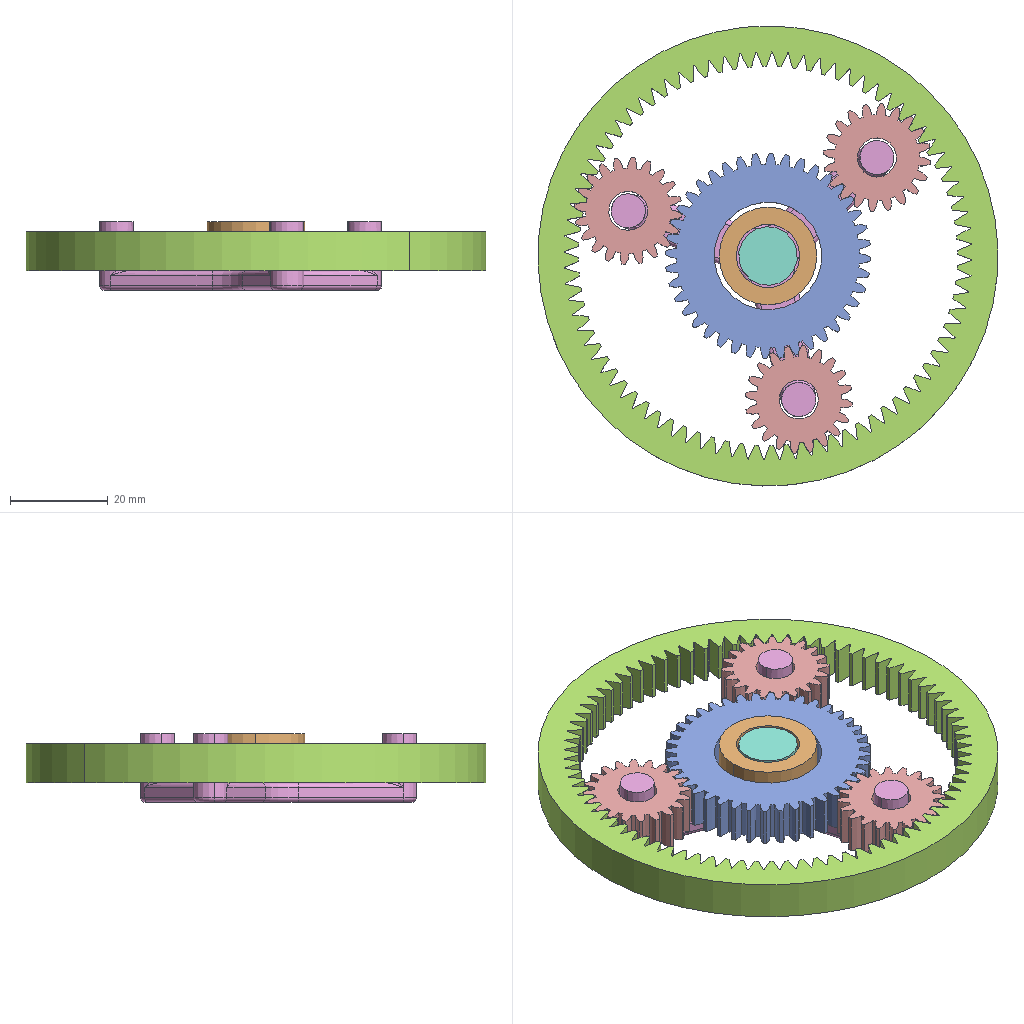Assembly | SolidWorks | 13 different items | 15 placed | box 94 x 94 x 14 mm
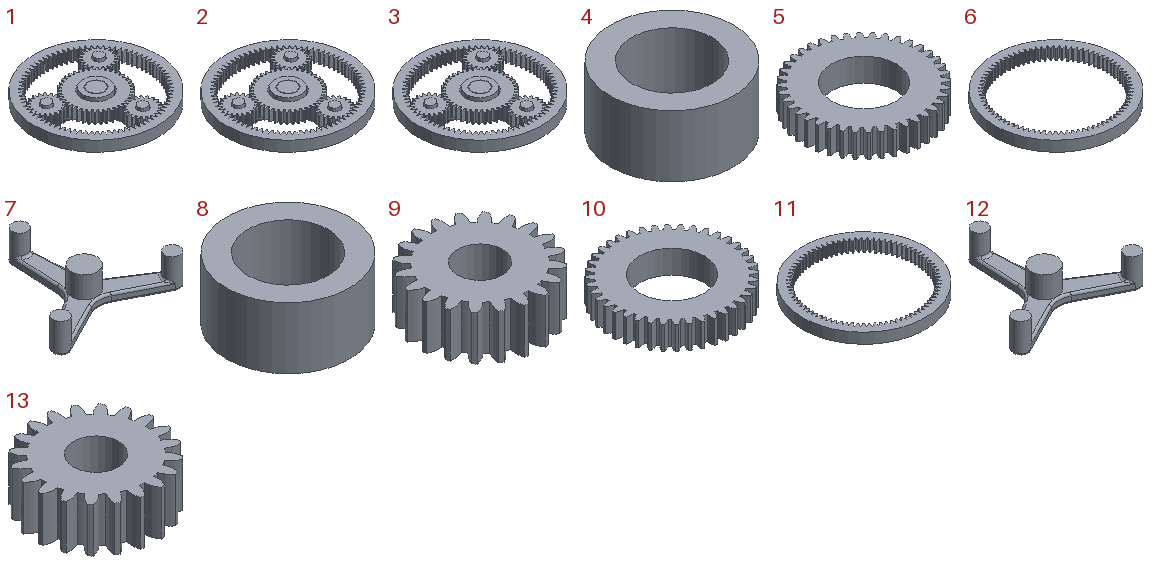Parts list (item | name | quantity | size | volume | features):
1 | (subassembly) | x1 | 94 x 94 x 14 mm | 35546 mm3 | features Attribute 48
2 | (subassembly) | x1 | 94 x 94 x 14 mm | 35546 mm3 | features Attribute 48
3 | (subassembly) | x1 | 94 x 94 x 14 mm | 35546 mm3 | features Attribute 48
4 | - | x1 | 20 x 20 x 10 mm | 1814 mm3 | features Cut 1, Extrusion 1
5 | - | x1 | 41.973 x 41.973 x 8 mm | 6925 mm3 | features Boss 1, CirPattern 1, Cut 1, Extrusion 1, RefAxis 1
6 | - | x1 | 94 x 94 x 8 mm | 15235 mm3 | features Cut 2, CirPattern 1, Extrusion 1, RefAxis 1
7 | - | x1 | 58.962 x 52 x 14 mm | 5388 mm3 | features Boss 1, Extrusion 1, Fillet 1
8 | - | x1 | 20 x 20 x 10 mm | 1814 mm3 | features Cut 1, Extrusion 1
9 | - | x1 | 21.958 x 21.958 x 8 mm | 2061 mm3 | features Boss 1, CirPattern 1, Cut 1, Extrusion 1, RefAxis 1
10 | - | x1 | 41.973 x 41.973 x 8 mm | 6925 mm3 | features Boss 1, CirPattern 1, Cut 1, Extrusion 1, RefAxis 1
11 | - | x1 | 94 x 94 x 8 mm | 15235 mm3 | features Cut 2, CirPattern 1, Extrusion 1, RefAxis 1
12 | - | x1 | 58.962 x 52 x 14 mm | 5388 mm3 | features Boss 1, Extrusion 1, Fillet 1
13 | - | x3 | 21.958 x 21.958 x 8 mm | 2061 mm3 | features Boss 1, CirPattern 1, Cut 1, Extrusion 1, RefAxis 1
Mates (type | each side: item.copy, entity, surface, feature):
Coincident | 5.1 face plane Extrude1 | 13.1 face plane Extrude1
Coincident | 13.2 face plane Extrude1 | 5.1 face plane Extrude1
Coincident | 5.1 face plane Extrude1 | 13.3 face plane Extrude1
Coincident | 5.1 face plane Extrude1 | 8.1 face plane Extrude1
Coincident | 5.1 face plane Extrude1 | 7.1 face plane Extrude2
Concentric | 5.1 face cylinder Cut-Extrude2 | 8.1 face cylinder Extrude1
Concentric | 6.1 face cylinder Extrude3 | 8.1 face cylinder Extrude1
Concentric | 13.2 face cylinder Cut-Extrude2 | 7.1 face cylinder Extrude1
Concentric | 13.1 face cylinder Cut-Extrude2 | 7.1 face cylinder Extrude1
Concentric | 13.3 face cylinder Cut-Extrude2 | 7.1 face cylinder Extrude1
Coincident | 5.1 face plane Extrude1 | 6.1 face plane Extrude3
Concentric | 7.1 face cylinder Extrude1 | 8.1 face cylinder Cut-Extrude1